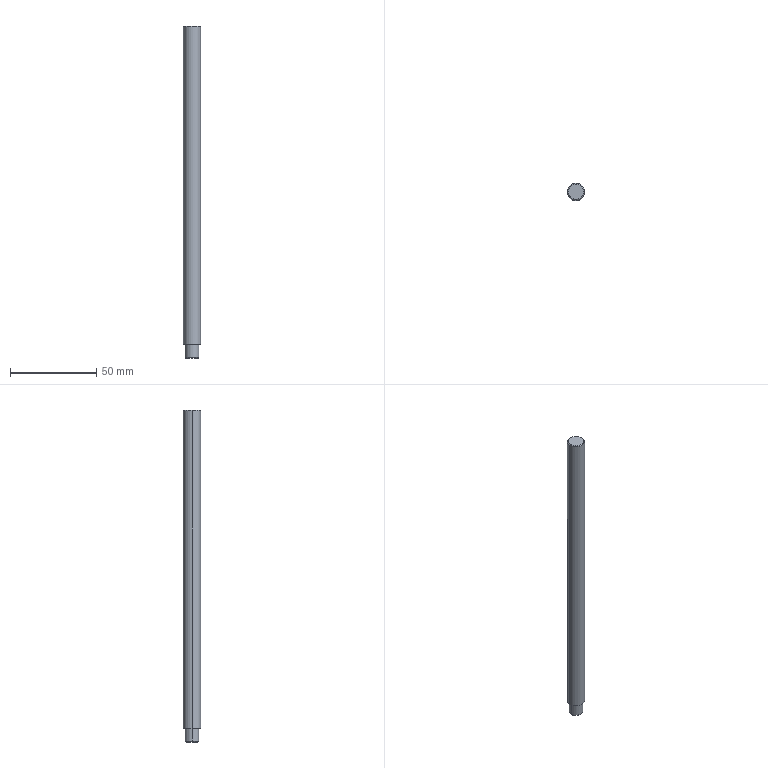Part | SolidWorks | features Chamfer 1, Extrusion 1, ICE 1 | 1 solid | 11 faces | box 10 x 10 x 193 mm | volume 14925 mm3 | cone 4 | cylinder 4 | plane 3 | commonest cylinder face diameters 8 x2 10 x2
STEP:
#1=CARTESIAN_POINT('',(4.5,0.,185.));
#2=VERTEX_POINT('',#1);
#3=CARTESIAN_POINT('',(-4.5,0.,185.));
#4=VERTEX_POINT('',#3);
#5=CARTESIAN_POINT('',(0.,0.,185.));
#6=DIRECTION('',(0.,0.,1.));
#7=DIRECTION('',(1.,0.,0.));
#8=AXIS2_PLACEMENT_3D('',#5,#6,#7);
#9=CIRCLE('',#8,4.5);
#10=EDGE_CURVE('',#2,#4,#9,.T.);
#11=ORIENTED_EDGE('',*,*,#10,.F.);
#12=CARTESIAN_POINT('',(5.,0.,184.5));
#13=VERTEX_POINT('',#12);
#14=CARTESIAN_POINT('',(4.5,0.,185.));
#15=DIRECTION('',(0.7071,0.,-0.7071));
#16=VECTOR('',#15,1000.);
#17=LINE('',#14,#16);
#18=EDGE_CURVE('',#2,#13,#17,.T.);
#19=ORIENTED_EDGE('',*,*,#18,.T.);
#20=CARTESIAN_POINT('',(-5.,0.,184.5));
#21=VERTEX_POINT('',#20);
#22=CARTESIAN_POINT('',(0.,0.,184.5));
#23=DIRECTION('',(0.,0.,-1.));
#24=DIRECTION('',(1.,0.,0.));
#25=AXIS2_PLACEMENT_3D('',#22,#23,#24);
#26=CIRCLE('',#25,5.);
#27=EDGE_CURVE('',#21,#13,#26,.T.);
#28=ORIENTED_EDGE('',*,*,#27,.F.);
#29=CARTESIAN_POINT('',(-4.5,0.,185.));
#30=DIRECTION('',(-0.7071,0.,-0.7071));
#31=VECTOR('',#30,1000.);
#32=LINE('',#29,#31);
#33=EDGE_CURVE('',#4,#21,#32,.T.);
#34=ORIENTED_EDGE('',*,*,#33,.F.);
#35=EDGE_LOOP('',(#11,#19,#28,#34));
#36=FACE_OUTER_BOUND('',#35,.T.);
#37=CARTESIAN_POINT('',(0.,0.,185.));
#38=DIRECTION('',(0.,0.,-1.));
#39=DIRECTION('',(-1.,0.,0.));
#40=AXIS2_PLACEMENT_3D('',#37,#38,#39);
#41=CONICAL_SURFACE('',#40,4.5,0.7854);
#42=ADVANCED_FACE('',(#36),#41,.T.);
#43=CARTESIAN_POINT('',(-3.5,0.,-8.));
#44=VERTEX_POINT('',#43);
#45=CARTESIAN_POINT('',(3.5,0.,-8.));
#46=VERTEX_POINT('',#45);
#47=CARTESIAN_POINT('',(0.,0.,-8.));
#48=DIRECTION('',(0.,0.,-1.));
#49=DIRECTION('',(-1.,0.,0.));
#50=AXIS2_PLACEMENT_3D('',#47,#48,#49);
#51=CIRCLE('',#50,3.5);
#52=EDGE_CURVE('',#44,#46,#51,.T.);
#53=ORIENTED_EDGE('',*,*,#52,.F.);
#54=CARTESIAN_POINT('',(-4.,0.,-7.5));
#55=VERTEX_POINT('',#54);
#56=CARTESIAN_POINT('',(-3.5,0.,-8.));
#57=DIRECTION('',(-0.7071,0.,0.7071));
#58=VECTOR('',#57,1000.);
#59=LINE('',#56,#58);
#60=EDGE_CURVE('',#44,#55,#59,.T.);
#61=ORIENTED_EDGE('',*,*,#60,.T.);
#62=CARTESIAN_POINT('',(4.,0.,-7.5));
#63=VERTEX_POINT('',#62);
#64=CARTESIAN_POINT('',(0.,0.,-7.5));
#65=DIRECTION('',(0.,0.,1.));
#66=DIRECTION('',(-1.,0.,0.));
#67=AXIS2_PLACEMENT_3D('',#64,#65,#66);
#68=CIRCLE('',#67,4.);
#69=EDGE_CURVE('',#63,#55,#68,.T.);
#70=ORIENTED_EDGE('',*,*,#69,.F.);
#71=CARTESIAN_POINT('',(3.5,0.,-8.));
#72=DIRECTION('',(0.7071,0.,0.7071));
#73=VECTOR('',#72,1000.);
#74=LINE('',#71,#73);
#75=EDGE_CURVE('',#46,#63,#74,.T.);
#76=ORIENTED_EDGE('',*,*,#75,.F.);
#77=EDGE_LOOP('',(#53,#61,#70,#76));
#78=FACE_OUTER_BOUND('',#77,.T.);
#79=CARTESIAN_POINT('',(0.,0.,-8.));
#80=DIRECTION('',(0.,0.,1.));
#81=DIRECTION('',(1.,0.,0.));
#82=AXIS2_PLACEMENT_3D('',#79,#80,#81);
#83=CONICAL_SURFACE('',#82,3.5,0.7854);
#84=ADVANCED_FACE('',(#78),#83,.T.);
#85=ORIENTED_EDGE('',*,*,#69,.T.);
#86=CARTESIAN_POINT('',(-4.,0.,0.));
#87=VERTEX_POINT('',#86);
#88=CARTESIAN_POINT('',(-4.,0.,-8.));
#89=DIRECTION('',(0.,0.,1.));
#90=VECTOR('',#89,1000.);
#91=LINE('',#88,#90);
#92=EDGE_CURVE('',#55,#87,#91,.T.);
#93=ORIENTED_EDGE('',*,*,#92,.T.);
#94=CARTESIAN_POINT('',(4.,0.,0.));
#95=VERTEX_POINT('',#94);
#96=CARTESIAN_POINT('',(0.,0.,0.));
#97=DIRECTION('',(0.,0.,-1.));
#98=DIRECTION('',(1.,0.,0.));
#99=AXIS2_PLACEMENT_3D('',#96,#97,#98);
#100=CIRCLE('',#99,4.);
#101=EDGE_CURVE('',#87,#95,#100,.T.);
#102=ORIENTED_EDGE('',*,*,#101,.T.);
#103=CARTESIAN_POINT('',(4.,0.,-8.));
#104=DIRECTION('',(0.,0.,1.));
#105=VECTOR('',#104,1000.);
#106=LINE('',#103,#105);
#107=EDGE_CURVE('',#63,#95,#106,.T.);
#108=ORIENTED_EDGE('',*,*,#107,.F.);
#109=EDGE_LOOP('',(#85,#93,#102,#108));
#110=FACE_OUTER_BOUND('',#109,.T.);
#111=CARTESIAN_POINT('',(0.,0.,-8.));
#112=DIRECTION('',(0.,0.,1.));
#113=DIRECTION('',(1.,0.,0.));
#114=AXIS2_PLACEMENT_3D('',#111,#112,#113);
#115=CYLINDRICAL_SURFACE('',#114,4.);
#116=ADVANCED_FACE('',(#110),#115,.T.);
#117=ORIENTED_EDGE('',*,*,#27,.T.);
#118=CARTESIAN_POINT('',(5.,0.,0.));
#119=VERTEX_POINT('',#118);
#120=CARTESIAN_POINT('',(5.,0.,185.));
#121=DIRECTION('',(0.,0.,-1.));
#122=VECTOR('',#121,1000.);
#123=LINE('',#120,#122);
#124=EDGE_CURVE('',#13,#119,#123,.T.);
#125=ORIENTED_EDGE('',*,*,#124,.T.);
#126=CARTESIAN_POINT('',(-5.,0.,0.));
#127=VERTEX_POINT('',#126);
#128=CARTESIAN_POINT('',(0.,0.,0.));
#129=DIRECTION('',(0.,0.,1.));
#130=DIRECTION('',(1.,0.,0.));
#131=AXIS2_PLACEMENT_3D('',#128,#129,#130);
#132=CIRCLE('',#131,5.);
#133=EDGE_CURVE('',#119,#127,#132,.T.);
#134=ORIENTED_EDGE('',*,*,#133,.T.);
#135=CARTESIAN_POINT('',(-5.,0.,185.));
#136=DIRECTION('',(0.,0.,-1.));
#137=VECTOR('',#136,1000.);
#138=LINE('',#135,#137);
#139=EDGE_CURVE('',#21,#127,#138,.T.);
#140=ORIENTED_EDGE('',*,*,#139,.F.);
#141=EDGE_LOOP('',(#117,#125,#134,#140));
#142=FACE_OUTER_BOUND('',#141,.T.);
#143=CARTESIAN_POINT('',(0.,0.,185.));
#144=DIRECTION('',(0.,0.,-1.));
#145=DIRECTION('',(-1.,0.,0.));
#146=AXIS2_PLACEMENT_3D('',#143,#144,#145);
#147=CYLINDRICAL_SURFACE('',#146,5.);
#148=ADVANCED_FACE('',(#142),#147,.T.);
#149=ORIENTED_EDGE('',*,*,#124,.F.);
#150=CARTESIAN_POINT('',(0.,0.,184.5));
#151=DIRECTION('',(0.,0.,-1.));
#152=DIRECTION('',(1.,0.,0.));
#153=AXIS2_PLACEMENT_3D('',#150,#151,#152);
#154=CIRCLE('',#153,5.);
#155=EDGE_CURVE('',#13,#21,#154,.T.);
#156=ORIENTED_EDGE('',*,*,#155,.T.);
#157=ORIENTED_EDGE('',*,*,#139,.T.);
#158=CARTESIAN_POINT('',(0.,0.,0.));
#159=DIRECTION('',(0.,0.,1.));
#160=DIRECTION('',(1.,0.,0.));
#161=AXIS2_PLACEMENT_3D('',#158,#159,#160);
#162=CIRCLE('',#161,5.);
#163=EDGE_CURVE('',#127,#119,#162,.T.);
#164=ORIENTED_EDGE('',*,*,#163,.T.);
#165=EDGE_LOOP('',(#149,#156,#157,#164));
#166=FACE_OUTER_BOUND('',#165,.T.);
#167=CARTESIAN_POINT('',(0.,0.,185.));
#168=DIRECTION('',(0.,0.,-1.));
#169=DIRECTION('',(-1.,0.,0.));
#170=AXIS2_PLACEMENT_3D('',#167,#168,#169);
#171=CYLINDRICAL_SURFACE('',#170,5.);
#172=ADVANCED_FACE('',(#166),#171,.T.);
#173=CARTESIAN_POINT('',(0.,0.,185.));
#174=DIRECTION('',(0.,0.,1.));
#175=DIRECTION('',(1.,0.,0.));
#176=AXIS2_PLACEMENT_3D('',#173,#174,#175);
#177=CIRCLE('',#176,4.5);
#178=EDGE_CURVE('',#4,#2,#177,.T.);
#179=ORIENTED_EDGE('',*,*,#178,.T.);
#180=ORIENTED_EDGE('',*,*,#10,.T.);
#181=EDGE_LOOP('',(#179,#180));
#182=FACE_OUTER_BOUND('',#181,.T.);
#183=CARTESIAN_POINT('',(0.,0.,185.));
#184=DIRECTION('',(0.,0.,1.));
#185=DIRECTION('',(1.,0.,0.));
#186=AXIS2_PLACEMENT_3D('',#183,#184,#185);
#187=PLANE('',#186);
#188=ADVANCED_FACE('',(#182),#187,.T.);
#189=CARTESIAN_POINT('',(0.,0.,0.));
#190=DIRECTION('',(0.,0.,-1.));
#191=DIRECTION('',(1.,0.,0.));
#192=AXIS2_PLACEMENT_3D('',#189,#190,#191);
#193=CIRCLE('',#192,4.);
#194=EDGE_CURVE('',#95,#87,#193,.T.);
#195=ORIENTED_EDGE('',*,*,#194,.F.);
#196=ORIENTED_EDGE('',*,*,#101,.F.);
#197=EDGE_LOOP('',(#195,#196));
#198=FACE_BOUND('',#197,.T.);
#199=ORIENTED_EDGE('',*,*,#163,.F.);
#200=ORIENTED_EDGE('',*,*,#133,.F.);
#201=EDGE_LOOP('',(#199,#200));
#202=FACE_OUTER_BOUND('',#201,.T.);
#203=CARTESIAN_POINT('',(0.,0.,0.));
#204=DIRECTION('',(0.,0.,1.));
#205=DIRECTION('',(1.,0.,0.));
#206=AXIS2_PLACEMENT_3D('',#203,#204,#205);
#207=PLANE('',#206);
#208=ADVANCED_FACE('',(#198,#202),#207,.F.);
#209=ORIENTED_EDGE('',*,*,#92,.F.);
#210=CARTESIAN_POINT('',(0.,0.,-7.5));
#211=DIRECTION('',(0.,0.,1.));
#212=DIRECTION('',(-1.,0.,0.));
#213=AXIS2_PLACEMENT_3D('',#210,#211,#212);
#214=CIRCLE('',#213,4.);
#215=EDGE_CURVE('',#55,#63,#214,.T.);
#216=ORIENTED_EDGE('',*,*,#215,.T.);
#217=ORIENTED_EDGE('',*,*,#107,.T.);
#218=ORIENTED_EDGE('',*,*,#194,.T.);
#219=EDGE_LOOP('',(#209,#216,#217,#218));
#220=FACE_OUTER_BOUND('',#219,.T.);
#221=CARTESIAN_POINT('',(0.,0.,-8.));
#222=DIRECTION('',(0.,0.,1.));
#223=DIRECTION('',(1.,0.,0.));
#224=AXIS2_PLACEMENT_3D('',#221,#222,#223);
#225=CYLINDRICAL_SURFACE('',#224,4.);
#226=ADVANCED_FACE('',(#220),#225,.T.);
#227=CARTESIAN_POINT('',(0.,0.,-8.));
#228=DIRECTION('',(0.,0.,-1.));
#229=DIRECTION('',(-1.,0.,0.));
#230=AXIS2_PLACEMENT_3D('',#227,#228,#229);
#231=CIRCLE('',#230,3.5);
#232=EDGE_CURVE('',#46,#44,#231,.T.);
#233=ORIENTED_EDGE('',*,*,#232,.T.);
#234=ORIENTED_EDGE('',*,*,#52,.T.);
#235=EDGE_LOOP('',(#233,#234));
#236=FACE_OUTER_BOUND('',#235,.T.);
#237=CARTESIAN_POINT('',(0.,0.,-8.));
#238=DIRECTION('',(0.,0.,-1.));
#239=DIRECTION('',(-1.,0.,0.));
#240=AXIS2_PLACEMENT_3D('',#237,#238,#239);
#241=PLANE('',#240);
#242=ADVANCED_FACE('',(#236),#241,.T.);
#243=ORIENTED_EDGE('',*,*,#60,.F.);
#244=ORIENTED_EDGE('',*,*,#232,.F.);
#245=ORIENTED_EDGE('',*,*,#75,.T.);
#246=ORIENTED_EDGE('',*,*,#215,.F.);
#247=EDGE_LOOP('',(#243,#244,#245,#246));
#248=FACE_OUTER_BOUND('',#247,.T.);
#249=CARTESIAN_POINT('',(0.,0.,-8.));
#250=DIRECTION('',(0.,0.,1.));
#251=DIRECTION('',(1.,0.,0.));
#252=AXIS2_PLACEMENT_3D('',#249,#250,#251);
#253=CONICAL_SURFACE('',#252,3.5,0.7854);
#254=ADVANCED_FACE('',(#248),#253,.T.);
#255=ORIENTED_EDGE('',*,*,#18,.F.);
#256=ORIENTED_EDGE('',*,*,#178,.F.);
#257=ORIENTED_EDGE('',*,*,#33,.T.);
#258=ORIENTED_EDGE('',*,*,#155,.F.);
#259=EDGE_LOOP('',(#255,#256,#257,#258));
#260=FACE_OUTER_BOUND('',#259,.T.);
#261=CARTESIAN_POINT('',(0.,0.,185.));
#262=DIRECTION('',(0.,0.,-1.));
#263=DIRECTION('',(-1.,0.,0.));
#264=AXIS2_PLACEMENT_3D('',#261,#262,#263);
#265=CONICAL_SURFACE('',#264,4.5,0.7854);
#266=ADVANCED_FACE('',(#260),#265,.T.);
#267=CLOSED_SHELL('',(#42,#84,#116,#148,#172,#188,#208,#226,#242,#254,#266));
#268=MANIFOLD_SOLID_BREP('',#267);
#269=CARTESIAN_POINT('',(0.,0.,0.));
#270=DIRECTION('',(0.,0.,1.));
#271=DIRECTION('',(1.,0.,0.));
#272=AXIS2_PLACEMENT_3D('',#269,#270,#271);
#273=(LENGTH_UNIT()NAMED_UNIT(*)SI_UNIT(.MILLI.,.METRE.));
#274=UNCERTAINTY_MEASURE_WITH_UNIT(LENGTH_MEASURE(0.00001),#273,'','');
#275=(NAMED_UNIT(*)PLANE_ANGLE_UNIT()SI_UNIT($,.RADIAN.));
#276=(NAMED_UNIT(*)SI_UNIT($,.STERADIAN.)SOLID_ANGLE_UNIT());
#277=(GEOMETRIC_REPRESENTATION_CONTEXT(3)GLOBAL_UNCERTAINTY_ASSIGNED_CONTEXT((#274))GLOBAL_UNIT_ASSIGNED_CONTEXT((#273,#275,#276))REPRESENTATION_CONTEXT('',''));
#278=ADVANCED_BREP_SHAPE_REPRESENTATION('',(#268,#272),#277);